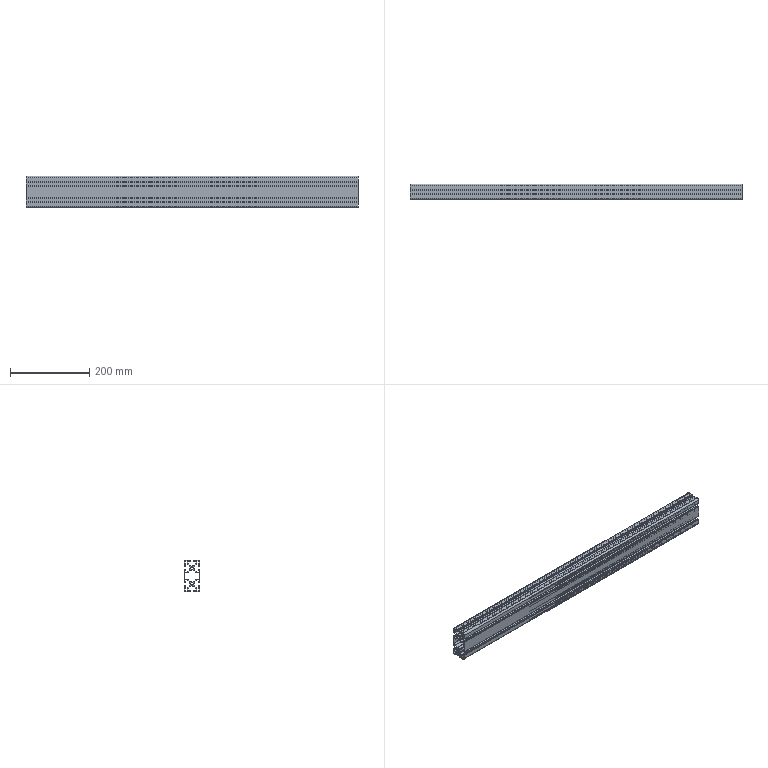Part | STEP file | 1 solid | 286 faces | box 840 x 40 x 80 mm | volume 681890 mm3 | cylinder 144 | plane 142 | commonest cylinder face diameters 0.6 x44 2 x44 4 x28 0.4 x14 6 x4 6.8 x4